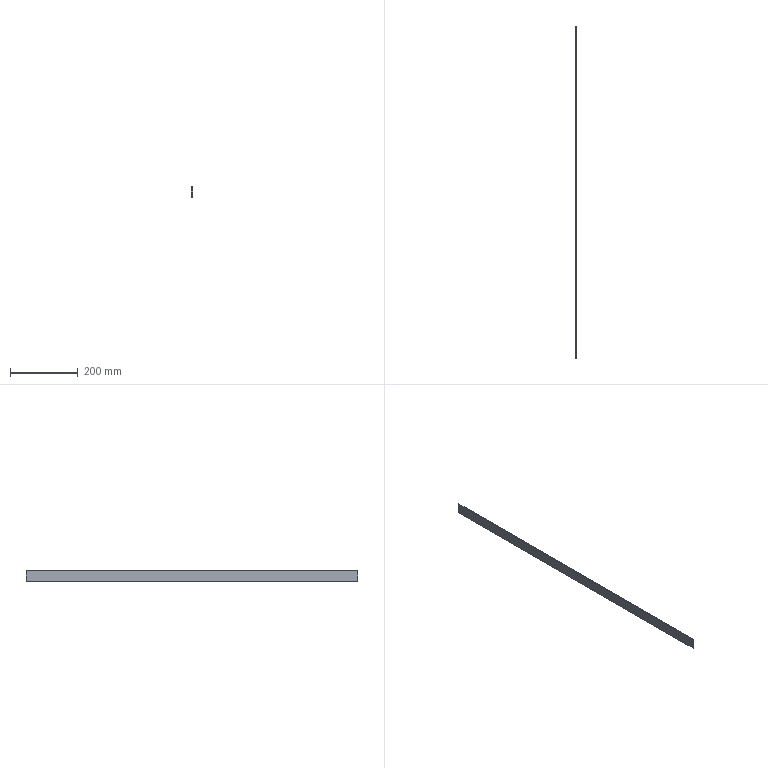Part | SolidWorks | 1 solid | 6 faces | box 3 x 980 x 30 mm | volume 88200 mm3 | plane 6
STEP:
#1=CARTESIAN_POINT('',(0.,490.,15.));
#2=VERTEX_POINT('',#1);
#3=CARTESIAN_POINT('',(0.,-490.,15.));
#4=VERTEX_POINT('',#3);
#5=CARTESIAN_POINT('',(0.,-490.,15.));
#6=DIRECTION('',(0.,-1.,0.));
#7=VECTOR('',#6,1000.);
#8=LINE('',#5,#7);
#9=EDGE_CURVE('',#2,#4,#8,.T.);
#10=ORIENTED_EDGE('',*,*,#9,.F.);
#11=CARTESIAN_POINT('',(-3.,490.,15.));
#12=VERTEX_POINT('',#11);
#13=CARTESIAN_POINT('',(-3.,490.,15.));
#14=DIRECTION('',(1.,0.,0.));
#15=VECTOR('',#14,1000.);
#16=LINE('',#13,#15);
#17=EDGE_CURVE('',#12,#2,#16,.T.);
#18=ORIENTED_EDGE('',*,*,#17,.F.);
#19=CARTESIAN_POINT('',(-3.,-490.,15.));
#20=VERTEX_POINT('',#19);
#21=CARTESIAN_POINT('',(-3.,-490.,15.));
#22=DIRECTION('',(0.,-1.,0.));
#23=VECTOR('',#22,1000.);
#24=LINE('',#21,#23);
#25=EDGE_CURVE('',#12,#20,#24,.T.);
#26=ORIENTED_EDGE('',*,*,#25,.T.);
#27=CARTESIAN_POINT('',(-3.,-490.,15.));
#28=DIRECTION('',(1.,0.,0.));
#29=VECTOR('',#28,1000.);
#30=LINE('',#27,#29);
#31=EDGE_CURVE('',#20,#4,#30,.T.);
#32=ORIENTED_EDGE('',*,*,#31,.T.);
#33=EDGE_LOOP('',(#10,#18,#26,#32));
#34=FACE_OUTER_BOUND('',#33,.T.);
#35=CARTESIAN_POINT('',(-3.,-490.,15.));
#36=DIRECTION('',(0.,0.,1.));
#37=DIRECTION('',(1.,0.,0.));
#38=AXIS2_PLACEMENT_3D('',#35,#36,#37);
#39=PLANE('',#38);
#40=ADVANCED_FACE('',(#34),#39,.T.);
#41=CARTESIAN_POINT('',(0.,490.,-15.));
#42=VERTEX_POINT('',#41);
#43=CARTESIAN_POINT('',(0.,490.,-15.));
#44=DIRECTION('',(0.,0.,1.));
#45=VECTOR('',#44,1000.);
#46=LINE('',#43,#45);
#47=EDGE_CURVE('',#42,#2,#46,.T.);
#48=ORIENTED_EDGE('',*,*,#47,.F.);
#49=CARTESIAN_POINT('',(-3.,490.,-15.));
#50=VERTEX_POINT('',#49);
#51=CARTESIAN_POINT('',(-3.,490.,-15.));
#52=DIRECTION('',(1.,0.,0.));
#53=VECTOR('',#52,1000.);
#54=LINE('',#51,#53);
#55=EDGE_CURVE('',#50,#42,#54,.T.);
#56=ORIENTED_EDGE('',*,*,#55,.F.);
#57=CARTESIAN_POINT('',(-3.,490.,-15.));
#58=DIRECTION('',(0.,0.,1.));
#59=VECTOR('',#58,1000.);
#60=LINE('',#57,#59);
#61=EDGE_CURVE('',#50,#12,#60,.T.);
#62=ORIENTED_EDGE('',*,*,#61,.T.);
#63=ORIENTED_EDGE('',*,*,#17,.T.);
#64=EDGE_LOOP('',(#48,#56,#62,#63));
#65=FACE_OUTER_BOUND('',#64,.T.);
#66=CARTESIAN_POINT('',(-3.,490.,-15.));
#67=DIRECTION('',(0.,1.,0.));
#68=DIRECTION('',(0.,0.,1.));
#69=AXIS2_PLACEMENT_3D('',#66,#67,#68);
#70=PLANE('',#69);
#71=ADVANCED_FACE('',(#65),#70,.T.);
#72=CARTESIAN_POINT('',(0.,-490.,-15.));
#73=VERTEX_POINT('',#72);
#74=CARTESIAN_POINT('',(0.,-490.,-15.));
#75=DIRECTION('',(0.,1.,0.));
#76=VECTOR('',#75,1000.);
#77=LINE('',#74,#76);
#78=EDGE_CURVE('',#73,#42,#77,.T.);
#79=ORIENTED_EDGE('',*,*,#78,.F.);
#80=CARTESIAN_POINT('',(-3.,-490.,-15.));
#81=VERTEX_POINT('',#80);
#82=CARTESIAN_POINT('',(-3.,-490.,-15.));
#83=DIRECTION('',(1.,0.,0.));
#84=VECTOR('',#83,1000.);
#85=LINE('',#82,#84);
#86=EDGE_CURVE('',#81,#73,#85,.T.);
#87=ORIENTED_EDGE('',*,*,#86,.F.);
#88=CARTESIAN_POINT('',(-3.,-490.,-15.));
#89=DIRECTION('',(0.,1.,0.));
#90=VECTOR('',#89,1000.);
#91=LINE('',#88,#90);
#92=EDGE_CURVE('',#81,#50,#91,.T.);
#93=ORIENTED_EDGE('',*,*,#92,.T.);
#94=ORIENTED_EDGE('',*,*,#55,.T.);
#95=EDGE_LOOP('',(#79,#87,#93,#94));
#96=FACE_OUTER_BOUND('',#95,.T.);
#97=CARTESIAN_POINT('',(-3.,-490.,-15.));
#98=DIRECTION('',(0.,0.,-1.));
#99=DIRECTION('',(-1.,0.,0.));
#100=AXIS2_PLACEMENT_3D('',#97,#98,#99);
#101=PLANE('',#100);
#102=ADVANCED_FACE('',(#96),#101,.T.);
#103=CARTESIAN_POINT('',(0.,-490.,-15.));
#104=DIRECTION('',(0.,0.,-1.));
#105=VECTOR('',#104,1000.);
#106=LINE('',#103,#105);
#107=EDGE_CURVE('',#4,#73,#106,.T.);
#108=ORIENTED_EDGE('',*,*,#107,.F.);
#109=ORIENTED_EDGE('',*,*,#31,.F.);
#110=CARTESIAN_POINT('',(-3.,-490.,-15.));
#111=DIRECTION('',(0.,0.,-1.));
#112=VECTOR('',#111,1000.);
#113=LINE('',#110,#112);
#114=EDGE_CURVE('',#20,#81,#113,.T.);
#115=ORIENTED_EDGE('',*,*,#114,.T.);
#116=ORIENTED_EDGE('',*,*,#86,.T.);
#117=EDGE_LOOP('',(#108,#109,#115,#116));
#118=FACE_OUTER_BOUND('',#117,.T.);
#119=CARTESIAN_POINT('',(-3.,-490.,-15.));
#120=DIRECTION('',(0.,-1.,0.));
#121=DIRECTION('',(0.,0.,-1.));
#122=AXIS2_PLACEMENT_3D('',#119,#120,#121);
#123=PLANE('',#122);
#124=ADVANCED_FACE('',(#118),#123,.T.);
#125=ORIENTED_EDGE('',*,*,#25,.F.);
#126=ORIENTED_EDGE('',*,*,#61,.F.);
#127=ORIENTED_EDGE('',*,*,#92,.F.);
#128=ORIENTED_EDGE('',*,*,#114,.F.);
#129=EDGE_LOOP('',(#125,#126,#127,#128));
#130=FACE_OUTER_BOUND('',#129,.T.);
#131=CARTESIAN_POINT('',(-3.,0.,0.));
#132=DIRECTION('',(1.,0.,0.));
#133=DIRECTION('',(0.,0.,-1.));
#134=AXIS2_PLACEMENT_3D('',#131,#132,#133);
#135=PLANE('',#134);
#136=ADVANCED_FACE('',(#130),#135,.F.);
#137=ORIENTED_EDGE('',*,*,#9,.T.);
#138=ORIENTED_EDGE('',*,*,#107,.T.);
#139=ORIENTED_EDGE('',*,*,#78,.T.);
#140=ORIENTED_EDGE('',*,*,#47,.T.);
#141=EDGE_LOOP('',(#137,#138,#139,#140));
#142=FACE_OUTER_BOUND('',#141,.T.);
#143=CARTESIAN_POINT('',(0.,0.,0.));
#144=DIRECTION('',(1.,0.,0.));
#145=DIRECTION('',(0.,0.,-1.));
#146=AXIS2_PLACEMENT_3D('',#143,#144,#145);
#147=PLANE('',#146);
#148=ADVANCED_FACE('',(#142),#147,.T.);
#149=CLOSED_SHELL('',(#40,#71,#102,#124,#136,#148));
#150=MANIFOLD_SOLID_BREP('',#149);
#151=CARTESIAN_POINT('',(0.,0.,0.));
#152=DIRECTION('',(0.,0.,1.));
#153=DIRECTION('',(1.,0.,0.));
#154=AXIS2_PLACEMENT_3D('',#151,#152,#153);
#155=(LENGTH_UNIT()NAMED_UNIT(*)SI_UNIT(.MILLI.,.METRE.));
#156=UNCERTAINTY_MEASURE_WITH_UNIT(LENGTH_MEASURE(0.00001),#155,'','');
#157=(NAMED_UNIT(*)PLANE_ANGLE_UNIT()SI_UNIT($,.RADIAN.));
#158=(NAMED_UNIT(*)SI_UNIT($,.STERADIAN.)SOLID_ANGLE_UNIT());
#159=(GEOMETRIC_REPRESENTATION_CONTEXT(3)GLOBAL_UNCERTAINTY_ASSIGNED_CONTEXT((#156))GLOBAL_UNIT_ASSIGNED_CONTEXT((#155,#157,#158))REPRESENTATION_CONTEXT('',''));
#160=ADVANCED_BREP_SHAPE_REPRESENTATION('',(#150,#154),#159);